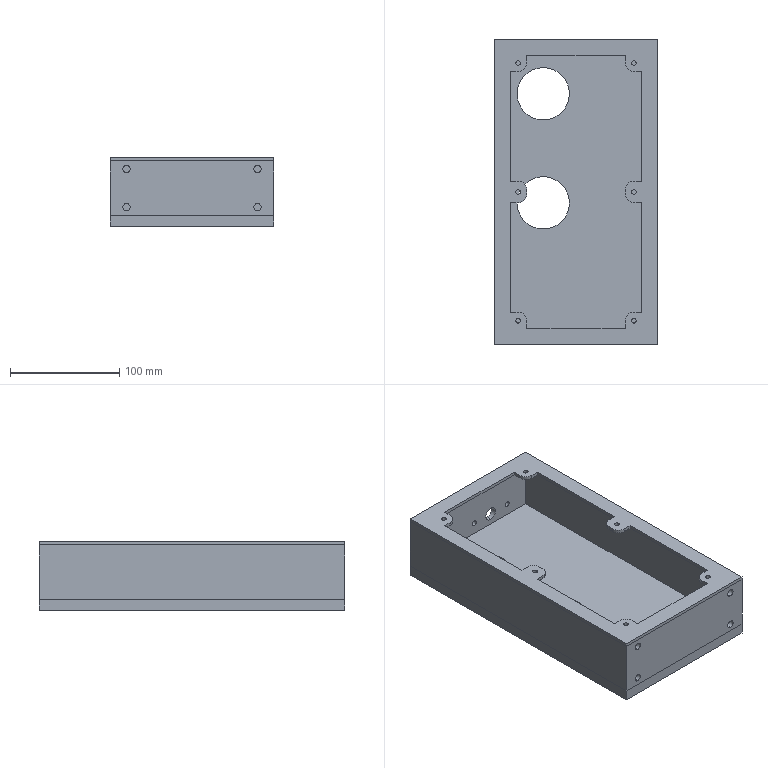Part | STEP file | Driven box QY-1-26 | 3 solids | 82 faces | box 150 x 280 x 63 mm | volume 632193 mm3 | plane 44 | cylinder 38 | commonest cylinder face diameters 4.2 x12 6.8 x8 16 x8 5 x4 48 x4 12.5 x2